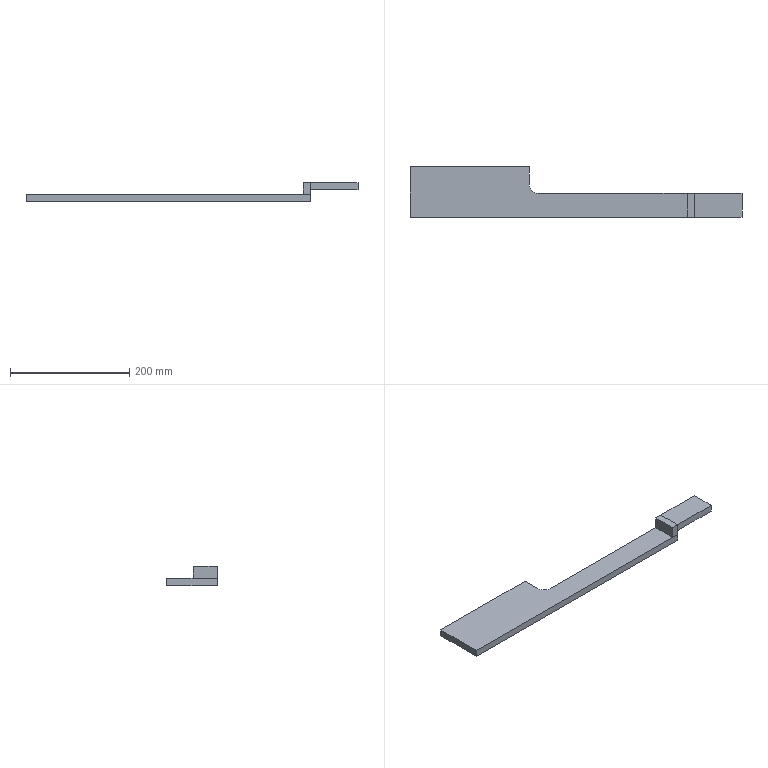Part | STEP file | PN_0035 | 1 solid | 17 faces | box 556.9 x 85 x 32 mm | volume 385323 mm3 | plane 16 | cylinder 1 | commonest cylinder face diameters 30 x1
STEP:
#1=CARTESIAN_POINT('',(0.,0.,0.));
#2=DIRECTION('',(0.,0.,1.));
#3=DIRECTION('',(1.,0.,0.));
#4=AXIS2_PLACEMENT_3D('',#1,#2,#3);
#5=CARTESIAN_POINT('',(238.4,-42.4,12.));
#6=VERTEX_POINT('',#5);
#7=CARTESIAN_POINT('',(238.4,-2.5,12.));
#8=VERTEX_POINT('',#7);
#9=CARTESIAN_POINT('',(238.4,42.4,12.));
#10=DIRECTION('',(0.,1.,0.));
#11=VECTOR('',#10,1.);
#12=LINE('',#9,#11);
#13=CARTESIAN_POINT('',(238.4,42.4,32.));
#14=DIRECTION('',(-1.,0.,0.));
#15=DIRECTION('',(0.,0.,1.));
#16=AXIS2_PLACEMENT_3D('',#13,#14,#15);
#17=PLANE('',#16);
#18=CARTESIAN_POINT('',(-20.,0.));
#19=DIRECTION('',(0.,1.));
#20=VECTOR('',#19,1.);
#21=LINE('',#18,#20);
#22=(GEOMETRIC_REPRESENTATION_CONTEXT(2)PARAMETRIC_REPRESENTATION_CONTEXT()REPRESENTATION_CONTEXT('',''));
#23=DEFINITIONAL_REPRESENTATION('',(#21),#22);
#24=PCURVE('',#17,#23);
#25=CARTESIAN_POINT('',(238.5,-42.5,12.));
#26=DIRECTION('',(0.,0.,1.));
#27=DIRECTION('',(1.,0.,0.));
#28=AXIS2_PLACEMENT_3D('',#25,#26,#27);
#29=PLANE('',#28);
#30=CARTESIAN_POINT('',(-0.1,84.9));
#31=DIRECTION('',(0.,1.));
#32=VECTOR('',#31,1.);
#33=LINE('',#30,#32);
#34=(GEOMETRIC_REPRESENTATION_CONTEXT(2)PARAMETRIC_REPRESENTATION_CONTEXT()REPRESENTATION_CONTEXT('',''));
#35=DEFINITIONAL_REPRESENTATION('',(#33),#34);
#36=PCURVE('',#29,#35);
#37=SURFACE_CURVE('',#12,(#24,#36),.PCURVE_S1.);
#38=EDGE_CURVE('',#6,#8,#37,.T.);
#39=ORIENTED_EDGE('',*,*,#38,.T.);
#40=CARTESIAN_POINT('',(238.4,-2.5,19.9));
#41=VERTEX_POINT('',#40);
#42=CARTESIAN_POINT('',(238.4,-2.5,32.));
#43=DIRECTION('',(0.,0.,1.));
#44=VECTOR('',#43,1.);
#45=LINE('',#42,#44);
#46=CARTESIAN_POINT('',(0.,-44.9));
#47=DIRECTION('',(1.,0.));
#48=VECTOR('',#47,1.);
#49=LINE('',#46,#48);
#50=(GEOMETRIC_REPRESENTATION_CONTEXT(2)PARAMETRIC_REPRESENTATION_CONTEXT()REPRESENTATION_CONTEXT('',''));
#51=DEFINITIONAL_REPRESENTATION('',(#49),#50);
#52=PCURVE('',#17,#51);
#53=CARTESIAN_POINT('',(-38.5,-2.5,32.));
#54=DIRECTION('',(0.,-1.,0.));
#55=DIRECTION('',(1.,0.,0.));
#56=AXIS2_PLACEMENT_3D('',#53,#54,#55);
#57=PLANE('',#56);
#58=CARTESIAN_POINT('',(276.9,0.));
#59=DIRECTION('',(0.,1.));
#60=VECTOR('',#59,1.);
#61=LINE('',#58,#60);
#62=(GEOMETRIC_REPRESENTATION_CONTEXT(2)PARAMETRIC_REPRESENTATION_CONTEXT()REPRESENTATION_CONTEXT('',''));
#63=DEFINITIONAL_REPRESENTATION('',(#61),#62);
#64=PCURVE('',#57,#63);
#65=SURFACE_CURVE('',#45,(#52,#64),.PCURVE_S1.);
#66=EDGE_CURVE('',#8,#41,#65,.T.);
#67=ORIENTED_EDGE('',*,*,#66,.T.);
#68=CARTESIAN_POINT('',(238.4,-42.3,19.9));
#69=VERTEX_POINT('',#68);
#70=CARTESIAN_POINT('',(238.4,42.3,19.9));
#71=DIRECTION('',(0.,1.,0.));
#72=VECTOR('',#71,1.);
#73=LINE('',#70,#72);
#74=CARTESIAN_POINT('',(-12.1,-0.1));
#75=DIRECTION('',(0.,1.));
#76=VECTOR('',#75,1.);
#77=LINE('',#74,#76);
#78=(GEOMETRIC_REPRESENTATION_CONTEXT(2)PARAMETRIC_REPRESENTATION_CONTEXT()REPRESENTATION_CONTEXT('',''));
#79=DEFINITIONAL_REPRESENTATION('',(#77),#78);
#80=PCURVE('',#17,#79);
#81=CARTESIAN_POINT('',(318.4,42.3,19.9));
#82=DIRECTION('',(0.,0.,1.));
#83=DIRECTION('',(0.,-1.,0.));
#84=AXIS2_PLACEMENT_3D('',#81,#82,#83);
#85=PLANE('',#84);
#86=CARTESIAN_POINT('',(0.,-80.));
#87=DIRECTION('',(-1.,0.));
#88=VECTOR('',#87,1.);
#89=LINE('',#86,#88);
#90=(GEOMETRIC_REPRESENTATION_CONTEXT(2)PARAMETRIC_REPRESENTATION_CONTEXT()REPRESENTATION_CONTEXT('',''));
#91=DEFINITIONAL_REPRESENTATION('',(#89),#90);
#92=PCURVE('',#85,#91);
#93=SURFACE_CURVE('',#73,(#80,#92),.PCURVE_S1.);
#94=EDGE_CURVE('',#69,#41,#93,.T.);
#95=ORIENTED_EDGE('',*,*,#94,.F.);
#96=CARTESIAN_POINT('',(238.4,-42.3,31.9));
#97=VERTEX_POINT('',#96);
#98=CARTESIAN_POINT('',(238.4,-42.3,31.9));
#99=DIRECTION('',(0.,0.,-1.));
#100=VECTOR('',#99,1.);
#101=LINE('',#98,#100);
#102=CARTESIAN_POINT('',(-0.1,-84.7));
#103=DIRECTION('',(-1.,0.));
#104=VECTOR('',#103,1.);
#105=LINE('',#102,#104);
#106=(GEOMETRIC_REPRESENTATION_CONTEXT(2)PARAMETRIC_REPRESENTATION_CONTEXT()REPRESENTATION_CONTEXT('',''));
#107=DEFINITIONAL_REPRESENTATION('',(#105),#106);
#108=PCURVE('',#17,#107);
#109=CARTESIAN_POINT('',(318.4,-42.3,31.9));
#110=DIRECTION('',(0.,1.,0.));
#111=DIRECTION('',(0.,0.,1.));
#112=AXIS2_PLACEMENT_3D('',#109,#110,#111);
#113=PLANE('',#112);
#114=CARTESIAN_POINT('',(0.,-80.));
#115=DIRECTION('',(-1.,0.));
#116=VECTOR('',#115,1.);
#117=LINE('',#114,#116);
#118=(GEOMETRIC_REPRESENTATION_CONTEXT(2)PARAMETRIC_REPRESENTATION_CONTEXT()REPRESENTATION_CONTEXT('',''));
#119=DEFINITIONAL_REPRESENTATION('',(#117),#118);
#120=PCURVE('',#113,#119);
#121=SURFACE_CURVE('',#101,(#108,#120),.PCURVE_S1.);
#122=EDGE_CURVE('',#97,#69,#121,.T.);
#123=ORIENTED_EDGE('',*,*,#122,.F.);
#124=CARTESIAN_POINT('',(238.4,-2.5,31.9));
#125=VERTEX_POINT('',#124);
#126=CARTESIAN_POINT('',(238.4,42.3,31.9));
#127=DIRECTION('',(0.,-1.,0.));
#128=VECTOR('',#127,1.);
#129=LINE('',#126,#128);
#130=CARTESIAN_POINT('',(-0.1,-0.1));
#131=DIRECTION('',(0.,-1.));
#132=VECTOR('',#131,1.);
#133=LINE('',#130,#132);
#134=(GEOMETRIC_REPRESENTATION_CONTEXT(2)PARAMETRIC_REPRESENTATION_CONTEXT()REPRESENTATION_CONTEXT('',''));
#135=DEFINITIONAL_REPRESENTATION('',(#133),#134);
#136=PCURVE('',#17,#135);
#137=CARTESIAN_POINT('',(318.4,42.3,31.9));
#138=DIRECTION('',(0.,0.,-1.));
#139=DIRECTION('',(0.,1.,0.));
#140=AXIS2_PLACEMENT_3D('',#137,#138,#139);
#141=PLANE('',#140);
#142=CARTESIAN_POINT('',(0.,-80.));
#143=DIRECTION('',(-1.,0.));
#144=VECTOR('',#143,1.);
#145=LINE('',#142,#144);
#146=(GEOMETRIC_REPRESENTATION_CONTEXT(2)PARAMETRIC_REPRESENTATION_CONTEXT()REPRESENTATION_CONTEXT('',''));
#147=DEFINITIONAL_REPRESENTATION('',(#145),#146);
#148=PCURVE('',#141,#147);
#149=SURFACE_CURVE('',#129,(#136,#148),.PCURVE_S1.);
#150=EDGE_CURVE('',#125,#97,#149,.T.);
#151=ORIENTED_EDGE('',*,*,#150,.F.);
#152=CARTESIAN_POINT('',(238.4,-2.5,32.));
#153=VERTEX_POINT('',#152);
#154=CARTESIAN_POINT('',(238.4,-2.5,32.));
#155=DIRECTION('',(0.,0.,1.));
#156=VECTOR('',#155,1.);
#157=LINE('',#154,#156);
#158=CARTESIAN_POINT('',(0.,-44.9));
#159=DIRECTION('',(1.,0.));
#160=VECTOR('',#159,1.);
#161=LINE('',#158,#160);
#162=(GEOMETRIC_REPRESENTATION_CONTEXT(2)PARAMETRIC_REPRESENTATION_CONTEXT()REPRESENTATION_CONTEXT('',''));
#163=DEFINITIONAL_REPRESENTATION('',(#161),#162);
#164=PCURVE('',#17,#163);
#165=CARTESIAN_POINT('',(276.9,0.));
#166=DIRECTION('',(0.,1.));
#167=VECTOR('',#166,1.);
#168=LINE('',#165,#167);
#169=(GEOMETRIC_REPRESENTATION_CONTEXT(2)PARAMETRIC_REPRESENTATION_CONTEXT()REPRESENTATION_CONTEXT('',''));
#170=DEFINITIONAL_REPRESENTATION('',(#168),#169);
#171=PCURVE('',#57,#170);
#172=SURFACE_CURVE('',#157,(#164,#171),.PCURVE_S1.);
#173=EDGE_CURVE('',#125,#153,#172,.T.);
#174=ORIENTED_EDGE('',*,*,#173,.T.);
#175=CARTESIAN_POINT('',(238.4,-42.4,32.));
#176=VERTEX_POINT('',#175);
#177=CARTESIAN_POINT('',(238.4,42.4,32.));
#178=DIRECTION('',(0.,1.,0.));
#179=VECTOR('',#178,1.);
#180=LINE('',#177,#179);
#181=CARTESIAN_POINT('',(0.,0.));
#182=DIRECTION('',(0.,1.));
#183=VECTOR('',#182,1.);
#184=LINE('',#181,#183);
#185=(GEOMETRIC_REPRESENTATION_CONTEXT(2)PARAMETRIC_REPRESENTATION_CONTEXT()REPRESENTATION_CONTEXT('',''));
#186=DEFINITIONAL_REPRESENTATION('',(#184),#185);
#187=PCURVE('',#17,#186);
#188=CARTESIAN_POINT('',(238.4,-42.4,32.));
#189=DIRECTION('',(0.,0.,-1.));
#190=DIRECTION('',(-1.,0.,0.));
#191=AXIS2_PLACEMENT_3D('',#188,#189,#190);
#192=PLANE('',#191);
#193=CARTESIAN_POINT('',(0.,84.8));
#194=DIRECTION('',(0.,1.));
#195=VECTOR('',#194,1.);
#196=LINE('',#193,#195);
#197=(GEOMETRIC_REPRESENTATION_CONTEXT(2)PARAMETRIC_REPRESENTATION_CONTEXT()REPRESENTATION_CONTEXT('',''));
#198=DEFINITIONAL_REPRESENTATION('',(#196),#197);
#199=PCURVE('',#192,#198);
#200=SURFACE_CURVE('',#180,(#187,#199),.PCURVE_S1.);
#201=EDGE_CURVE('',#176,#153,#200,.T.);
#202=ORIENTED_EDGE('',*,*,#201,.F.);
#203=CARTESIAN_POINT('',(238.4,-42.4,32.));
#204=DIRECTION('',(0.,0.,-1.));
#205=VECTOR('',#204,1.);
#206=LINE('',#203,#205);
#207=CARTESIAN_POINT('',(0.,-84.8));
#208=DIRECTION('',(-1.,0.));
#209=VECTOR('',#208,1.);
#210=LINE('',#207,#209);
#211=(GEOMETRIC_REPRESENTATION_CONTEXT(2)PARAMETRIC_REPRESENTATION_CONTEXT()REPRESENTATION_CONTEXT('',''));
#212=DEFINITIONAL_REPRESENTATION('',(#210),#211);
#213=PCURVE('',#17,#212);
#214=CARTESIAN_POINT('',(238.4,-42.4,32.));
#215=DIRECTION('',(0.,1.,0.));
#216=DIRECTION('',(0.,0.,1.));
#217=AXIS2_PLACEMENT_3D('',#214,#215,#216);
#218=PLANE('',#217);
#219=CARTESIAN_POINT('',(0.,0.));
#220=DIRECTION('',(-1.,0.));
#221=VECTOR('',#220,1.);
#222=LINE('',#219,#221);
#223=(GEOMETRIC_REPRESENTATION_CONTEXT(2)PARAMETRIC_REPRESENTATION_CONTEXT()REPRESENTATION_CONTEXT('',''));
#224=DEFINITIONAL_REPRESENTATION('',(#222),#223);
#225=PCURVE('',#218,#224);
#226=SURFACE_CURVE('',#206,(#213,#225),.PCURVE_S1.);
#227=EDGE_CURVE('',#176,#6,#226,.T.);
#228=ORIENTED_EDGE('',*,*,#227,.T.);
#229=EDGE_LOOP('',(#39,#67,#95,#123,#151,#174,#202,#228));
#230=FACE_BOUND('',#229,.T.);
#231=ADVANCED_FACE('',(#230),#17,.F.);
#232=CARTESIAN_POINT('',(-38.5,42.5,12.));
#233=VERTEX_POINT('',#232);
#234=CARTESIAN_POINT('',(-38.5,12.5,12.));
#235=VERTEX_POINT('',#234);
#236=CARTESIAN_POINT('',(-38.5,-42.5,12.));
#237=DIRECTION('',(0.,-1.,0.));
#238=VECTOR('',#237,1.);
#239=LINE('',#236,#238);
#240=CARTESIAN_POINT('',(-277.,0.));
#241=DIRECTION('',(0.,-1.));
#242=VECTOR('',#241,1.);
#243=LINE('',#240,#242);
#244=(GEOMETRIC_REPRESENTATION_CONTEXT(2)PARAMETRIC_REPRESENTATION_CONTEXT()REPRESENTATION_CONTEXT('',''));
#245=DEFINITIONAL_REPRESENTATION('',(#243),#244);
#246=PCURVE('',#29,#245);
#247=CARTESIAN_POINT('',(-38.5,42.5,32.));
#248=DIRECTION('',(-1.,0.,0.));
#249=DIRECTION('',(0.,-1.,0.));
#250=AXIS2_PLACEMENT_3D('',#247,#248,#249);
#251=PLANE('',#250);
#252=CARTESIAN_POINT('',(85.,-20.));
#253=DIRECTION('',(1.,0.));
#254=VECTOR('',#253,1.);
#255=LINE('',#252,#254);
#256=(GEOMETRIC_REPRESENTATION_CONTEXT(2)PARAMETRIC_REPRESENTATION_CONTEXT()REPRESENTATION_CONTEXT('',''));
#257=DEFINITIONAL_REPRESENTATION('',(#255),#256);
#258=PCURVE('',#251,#257);
#259=SURFACE_CURVE('',#239,(#246,#258),.PCURVE_S1.);
#260=EDGE_CURVE('',#233,#235,#259,.T.);
#261=ORIENTED_EDGE('',*,*,#260,.F.);
#262=CARTESIAN_POINT('',(-238.5,42.5,12.));
#263=VERTEX_POINT('',#262);
#264=CARTESIAN_POINT('',(-238.5,42.5,12.));
#265=DIRECTION('',(-1.,0.,0.));
#266=VECTOR('',#265,1.);
#267=LINE('',#264,#266);
#268=CARTESIAN_POINT('',(-477.,85.));
#269=DIRECTION('',(-1.,0.));
#270=VECTOR('',#269,1.);
#271=LINE('',#268,#270);
#272=(GEOMETRIC_REPRESENTATION_CONTEXT(2)PARAMETRIC_REPRESENTATION_CONTEXT()REPRESENTATION_CONTEXT('',''));
#273=DEFINITIONAL_REPRESENTATION('',(#271),#272);
#274=PCURVE('',#29,#273);
#275=CARTESIAN_POINT('',(-238.5,42.5,12.));
#276=DIRECTION('',(0.,-1.,0.));
#277=DIRECTION('',(0.,0.,-1.));
#278=AXIS2_PLACEMENT_3D('',#275,#276,#277);
#279=PLANE('',#278);
#280=CARTESIAN_POINT('',(0.,0.));
#281=DIRECTION('',(0.,-1.));
#282=VECTOR('',#281,1.);
#283=LINE('',#280,#282);
#284=(GEOMETRIC_REPRESENTATION_CONTEXT(2)PARAMETRIC_REPRESENTATION_CONTEXT()REPRESENTATION_CONTEXT('',''));
#285=DEFINITIONAL_REPRESENTATION('',(#283),#284);
#286=PCURVE('',#279,#285);
#287=SURFACE_CURVE('',#267,(#274,#286),.PCURVE_S1.);
#288=EDGE_CURVE('',#233,#263,#287,.T.);
#289=ORIENTED_EDGE('',*,*,#288,.T.);
#290=CARTESIAN_POINT('',(-238.5,-42.5,12.));
#291=VERTEX_POINT('',#290);
#292=CARTESIAN_POINT('',(-238.5,42.5,12.));
#293=DIRECTION('',(0.,-1.,0.));
#294=VECTOR('',#293,1.);
#295=LINE('',#292,#294);
#296=CARTESIAN_POINT('',(-477.,85.));
#297=DIRECTION('',(0.,-1.));
#298=VECTOR('',#297,1.);
#299=LINE('',#296,#298);
#300=(GEOMETRIC_REPRESENTATION_CONTEXT(2)PARAMETRIC_REPRESENTATION_CONTEXT()REPRESENTATION_CONTEXT('',''));
#301=DEFINITIONAL_REPRESENTATION('',(#299),#300);
#302=PCURVE('',#29,#301);
#303=CARTESIAN_POINT('',(-238.5,42.5,12.));
#304=DIRECTION('',(1.,0.,0.));
#305=DIRECTION('',(0.,0.,-1.));
#306=AXIS2_PLACEMENT_3D('',#303,#304,#305);
#307=PLANE('',#306);
#308=CARTESIAN_POINT('',(0.,0.));
#309=DIRECTION('',(0.,-1.));
#310=VECTOR('',#309,1.);
#311=LINE('',#308,#310);
#312=(GEOMETRIC_REPRESENTATION_CONTEXT(2)PARAMETRIC_REPRESENTATION_CONTEXT()REPRESENTATION_CONTEXT('',''));
#313=DEFINITIONAL_REPRESENTATION('',(#311),#312);
#314=PCURVE('',#307,#313);
#315=SURFACE_CURVE('',#295,(#302,#314),.PCURVE_S1.);
#316=EDGE_CURVE('',#263,#291,#315,.T.);
#317=ORIENTED_EDGE('',*,*,#316,.T.);
#318=CARTESIAN_POINT('',(238.5,-42.5,12.));
#319=VERTEX_POINT('',#318);
#320=CARTESIAN_POINT('',(-238.5,-42.5,12.));
#321=DIRECTION('',(1.,0.,0.));
#322=VECTOR('',#321,1.);
#323=LINE('',#320,#322);
#324=CARTESIAN_POINT('',(-477.,0.));
#325=DIRECTION('',(1.,0.));
#326=VECTOR('',#325,1.);
#327=LINE('',#324,#326);
#328=(GEOMETRIC_REPRESENTATION_CONTEXT(2)PARAMETRIC_REPRESENTATION_CONTEXT()REPRESENTATION_CONTEXT('',''));
#329=DEFINITIONAL_REPRESENTATION('',(#327),#328);
#330=PCURVE('',#29,#329);
#331=CARTESIAN_POINT('',(-238.5,-42.5,12.));
#332=DIRECTION('',(0.,1.,0.));
#333=DIRECTION('',(0.,0.,1.));
#334=AXIS2_PLACEMENT_3D('',#331,#332,#333);
#335=PLANE('',#334);
#336=CARTESIAN_POINT('',(0.,0.));
#337=DIRECTION('',(0.,1.));
#338=VECTOR('',#337,1.);
#339=LINE('',#336,#338);
#340=(GEOMETRIC_REPRESENTATION_CONTEXT(2)PARAMETRIC_REPRESENTATION_CONTEXT()REPRESENTATION_CONTEXT('',''));
#341=DEFINITIONAL_REPRESENTATION('',(#339),#340);
#342=PCURVE('',#335,#341);
#343=SURFACE_CURVE('',#323,(#330,#342),.PCURVE_S1.);
#344=EDGE_CURVE('',#291,#319,#343,.T.);
#345=ORIENTED_EDGE('',*,*,#344,.T.);
#346=CARTESIAN_POINT('',(238.5,-2.5,12.));
#347=VERTEX_POINT('',#346);
#348=CARTESIAN_POINT('',(238.5,42.5,12.));
#349=DIRECTION('',(0.,1.,0.));
#350=VECTOR('',#349,1.);
#351=LINE('',#348,#350);
#352=CARTESIAN_POINT('',(0.,85.));
#353=DIRECTION('',(0.,1.));
#354=VECTOR('',#353,1.);
#355=LINE('',#352,#354);
#356=(GEOMETRIC_REPRESENTATION_CONTEXT(2)PARAMETRIC_REPRESENTATION_CONTEXT()REPRESENTATION_CONTEXT('',''));
#357=DEFINITIONAL_REPRESENTATION('',(#355),#356);
#358=PCURVE('',#29,#357);
#359=CARTESIAN_POINT('',(238.5,42.5,12.));
#360=DIRECTION('',(-1.,0.,0.));
#361=DIRECTION('',(0.,-1.,0.));
#362=AXIS2_PLACEMENT_3D('',#359,#360,#361);
#363=PLANE('',#362);
#364=CARTESIAN_POINT('',(0.,0.));
#365=DIRECTION('',(-1.,0.));
#366=VECTOR('',#365,1.);
#367=LINE('',#364,#366);
#368=(GEOMETRIC_REPRESENTATION_CONTEXT(2)PARAMETRIC_REPRESENTATION_CONTEXT()REPRESENTATION_CONTEXT('',''));
#369=DEFINITIONAL_REPRESENTATION('',(#367),#368);
#370=PCURVE('',#363,#369);
#371=SURFACE_CURVE('',#351,(#358,#370),.PCURVE_S1.);
#372=EDGE_CURVE('',#319,#347,#371,.T.);
#373=ORIENTED_EDGE('',*,*,#372,.T.);
#374=CARTESIAN_POINT('',(238.5,-2.5,12.));
#375=DIRECTION('',(1.,0.,0.));
#376=VECTOR('',#375,1.);
#377=LINE('',#374,#376);
#378=CARTESIAN_POINT('',(0.,40.));
#379=DIRECTION('',(1.,0.));
#380=VECTOR('',#379,1.);
#381=LINE('',#378,#380);
#382=(GEOMETRIC_REPRESENTATION_CONTEXT(2)PARAMETRIC_REPRESENTATION_CONTEXT()REPRESENTATION_CONTEXT('',''));
#383=DEFINITIONAL_REPRESENTATION('',(#381),#382);
#384=PCURVE('',#29,#383);
#385=CARTESIAN_POINT('',(277.,-20.));
#386=DIRECTION('',(1.,0.));
#387=VECTOR('',#386,1.);
#388=LINE('',#385,#387);
#389=(GEOMETRIC_REPRESENTATION_CONTEXT(2)PARAMETRIC_REPRESENTATION_CONTEXT()REPRESENTATION_CONTEXT('',''));
#390=DEFINITIONAL_REPRESENTATION('',(#388),#389);
#391=PCURVE('',#57,#390);
#392=SURFACE_CURVE('',#377,(#384,#391),.PCURVE_S1.);
#393=EDGE_CURVE('',#8,#347,#392,.T.);
#394=ORIENTED_EDGE('',*,*,#393,.F.);
#395=ORIENTED_EDGE('',*,*,#38,.F.);
#396=CARTESIAN_POINT('',(226.4,-42.4,12.));
#397=VERTEX_POINT('',#396);
#398=CARTESIAN_POINT('',(238.4,-42.4,12.));
#399=DIRECTION('',(1.,0.,0.));
#400=VECTOR('',#399,1.);
#401=LINE('',#398,#400);
#402=CARTESIAN_POINT('',(-0.1,0.1));
#403=DIRECTION('',(1.,0.));
#404=VECTOR('',#403,1.);
#405=LINE('',#402,#404);
#406=(GEOMETRIC_REPRESENTATION_CONTEXT(2)PARAMETRIC_REPRESENTATION_CONTEXT()REPRESENTATION_CONTEXT('',''));
#407=DEFINITIONAL_REPRESENTATION('',(#405),#406);
#408=PCURVE('',#29,#407);
#409=CARTESIAN_POINT('',(-20.,0.));
#410=DIRECTION('',(0.,1.));
#411=VECTOR('',#410,1.);
#412=LINE('',#409,#411);
#413=(GEOMETRIC_REPRESENTATION_CONTEXT(2)PARAMETRIC_REPRESENTATION_CONTEXT()REPRESENTATION_CONTEXT('',''));
#414=DEFINITIONAL_REPRESENTATION('',(#412),#413);
#415=PCURVE('',#218,#414);
#416=SURFACE_CURVE('',#401,(#408,#415),.PCURVE_S1.);
#417=EDGE_CURVE('',#397,#6,#416,.T.);
#418=ORIENTED_EDGE('',*,*,#417,.F.);
#419=CARTESIAN_POINT('',(226.4,-2.5,12.));
#420=VERTEX_POINT('',#419);
#421=CARTESIAN_POINT('',(226.4,42.4,12.));
#422=DIRECTION('',(0.,-1.,0.));
#423=VECTOR('',#422,1.);
#424=LINE('',#421,#423);
#425=CARTESIAN_POINT('',(-12.1,84.9));
#426=DIRECTION('',(0.,-1.));
#427=VECTOR('',#426,1.);
#428=LINE('',#425,#427);
#429=(GEOMETRIC_REPRESENTATION_CONTEXT(2)PARAMETRIC_REPRESENTATION_CONTEXT()REPRESENTATION_CONTEXT('',''));
#430=DEFINITIONAL_REPRESENTATION('',(#428),#429);
#431=PCURVE('',#29,#430);
#432=CARTESIAN_POINT('',(226.4,42.4,32.));
#433=DIRECTION('',(1.,0.,0.));
#434=DIRECTION('',(0.,0.,-1.));
#435=AXIS2_PLACEMENT_3D('',#432,#433,#434);
#436=PLANE('',#435);
#437=CARTESIAN_POINT('',(20.,0.));
#438=DIRECTION('',(0.,-1.));
#439=VECTOR('',#438,1.);
#440=LINE('',#437,#439);
#441=(GEOMETRIC_REPRESENTATION_CONTEXT(2)PARAMETRIC_REPRESENTATION_CONTEXT()REPRESENTATION_CONTEXT('',''));
#442=DEFINITIONAL_REPRESENTATION('',(#440),#441);
#443=PCURVE('',#436,#442);
#444=SURFACE_CURVE('',#424,(#431,#443),.PCURVE_S1.);
#445=EDGE_CURVE('',#420,#397,#444,.T.);
#446=ORIENTED_EDGE('',*,*,#445,.F.);
#447=CARTESIAN_POINT('',(-23.5,-2.5,12.));
#448=VERTEX_POINT('',#447);
#449=CARTESIAN_POINT('',(238.5,-2.5,12.));
#450=DIRECTION('',(1.,0.,0.));
#451=VECTOR('',#450,1.);
#452=LINE('',#449,#451);
#453=CARTESIAN_POINT('',(0.,40.));
#454=DIRECTION('',(1.,0.));
#455=VECTOR('',#454,1.);
#456=LINE('',#453,#455);
#457=(GEOMETRIC_REPRESENTATION_CONTEXT(2)PARAMETRIC_REPRESENTATION_CONTEXT()REPRESENTATION_CONTEXT('',''));
#458=DEFINITIONAL_REPRESENTATION('',(#456),#457);
#459=PCURVE('',#29,#458);
#460=CARTESIAN_POINT('',(277.,-20.));
#461=DIRECTION('',(1.,0.));
#462=VECTOR('',#461,1.);
#463=LINE('',#460,#462);
#464=(GEOMETRIC_REPRESENTATION_CONTEXT(2)PARAMETRIC_REPRESENTATION_CONTEXT()REPRESENTATION_CONTEXT('',''));
#465=DEFINITIONAL_REPRESENTATION('',(#463),#464);
#466=PCURVE('',#57,#465);
#467=SURFACE_CURVE('',#452,(#459,#466),.PCURVE_S1.);
#468=EDGE_CURVE('',#448,#420,#467,.T.);
#469=ORIENTED_EDGE('',*,*,#468,.F.);
#470=CARTESIAN_POINT('',(-23.5,12.5,12.));
#471=DIRECTION('',(0.,0.,-1.));
#472=DIRECTION('',(1.,0.,0.));
#473=AXIS2_PLACEMENT_3D('',#470,#471,#472);
#474=CIRCLE('',#473,15.);
#475=CARTESIAN_POINT('',(-247.,55.));
#476=CARTESIAN_POINT('',(-247.,29.019));
#477=CARTESIAN_POINT('',(-269.5,42.01));
#478=CARTESIAN_POINT('',(-292.,55.));
#479=CARTESIAN_POINT('',(-269.5,67.99));
#480=CARTESIAN_POINT('',(-247.,80.981));
#481=CARTESIAN_POINT('',(-247.,55.));
#482=(BOUNDED_CURVE()B_SPLINE_CURVE(2,(#475,#476,#477,#478,#479,#480,#481),.UNSPECIFIED.,.T.,.F.)B_SPLINE_CURVE_WITH_KNOTS((1,2,2,2,2,1),(-2.094,0.,2.094,4.189,6.283,8.378),.UNSPECIFIED.)CURVE()GEOMETRIC_REPRESENTATION_ITEM()RATIONAL_B_SPLINE_CURVE((1.,0.5,1.,0.5,1.,0.5,1.))REPRESENTATION_ITEM(''));
#483=(GEOMETRIC_REPRESENTATION_CONTEXT(2)PARAMETRIC_REPRESENTATION_CONTEXT()REPRESENTATION_CONTEXT('',''));
#484=DEFINITIONAL_REPRESENTATION('',(#482),#483);
#485=PCURVE('',#29,#484);
#486=CARTESIAN_POINT('',(-23.5,12.5,32.));
#487=DIRECTION('',(0.,0.,1.));
#488=DIRECTION('',(1.,0.,0.));
#489=AXIS2_PLACEMENT_3D('',#486,#487,#488);
#490=CYLINDRICAL_SURFACE('',#489,15.);
#491=CARTESIAN_POINT('',(6.283,-20.));
#492=DIRECTION('',(-1.,0.));
#493=VECTOR('',#492,1.);
#494=LINE('',#491,#493);
#495=(GEOMETRIC_REPRESENTATION_CONTEXT(2)PARAMETRIC_REPRESENTATION_CONTEXT()REPRESENTATION_CONTEXT('',''));
#496=DEFINITIONAL_REPRESENTATION('',(#494),#495);
#497=PCURVE('',#490,#496);
#498=SURFACE_CURVE('',#474,(#485,#497),.PCURVE_S1.);
#499=EDGE_CURVE('',#448,#235,#498,.T.);
#500=ORIENTED_EDGE('',*,*,#499,.T.);
#501=EDGE_LOOP('',(#261,#289,#317,#345,#373,#394,#395,#418,#446,#469,#500));
#502=FACE_BOUND('',#501,.T.);
#503=ADVANCED_FACE('',(#502),#29,.T.);
#504=CARTESIAN_POINT('',(238.5,-42.5,0.));
#505=VERTEX_POINT('',#504);
#506=CARTESIAN_POINT('',(238.5,-2.5,0.));
#507=VERTEX_POINT('',#506);
#508=CARTESIAN_POINT('',(238.5,42.5,0.));
#509=DIRECTION('',(0.,1.,0.));
#510=VECTOR('',#509,1.);
#511=LINE('',#508,#510);
#512=CARTESIAN_POINT('',(0.,-12.));
#513=DIRECTION('',(-1.,0.));
#514=VECTOR('',#513,1.);
#515=LINE('',#512,#514);
#516=(GEOMETRIC_REPRESENTATION_CONTEXT(2)PARAMETRIC_REPRESENTATION_CONTEXT()REPRESENTATION_CONTEXT('',''));
#517=DEFINITIONAL_REPRESENTATION('',(#515),#516);
#518=PCURVE('',#363,#517);
#519=CARTESIAN_POINT('',(238.5,-42.5,0.));
#520=DIRECTION('',(0.,0.,1.));
#521=DIRECTION('',(1.,0.,0.));
#522=AXIS2_PLACEMENT_3D('',#519,#520,#521);
#523=PLANE('',#522);
#524=CARTESIAN_POINT('',(0.,85.));
#525=DIRECTION('',(0.,1.));
#526=VECTOR('',#525,1.);
#527=LINE('',#524,#526);
#528=(GEOMETRIC_REPRESENTATION_CONTEXT(2)PARAMETRIC_REPRESENTATION_CONTEXT()REPRESENTATION_CONTEXT('',''));
#529=DEFINITIONAL_REPRESENTATION('',(#527),#528);
#530=PCURVE('',#523,#529);
#531=SURFACE_CURVE('',#511,(#518,#530),.PCURVE_S1.);
#532=EDGE_CURVE('',#505,#507,#531,.T.);
#533=ORIENTED_EDGE('',*,*,#532,.T.);
#534=CARTESIAN_POINT('',(238.5,-2.5,12.));
#535=DIRECTION('',(0.,0.,1.));
#536=VECTOR('',#535,1.);
#537=LINE('',#534,#536);
#538=CARTESIAN_POINT('',(45.,0.));
#539=DIRECTION('',(0.,1.));
#540=VECTOR('',#539,1.);
#541=LINE('',#538,#540);
#542=(GEOMETRIC_REPRESENTATION_CONTEXT(2)PARAMETRIC_REPRESENTATION_CONTEXT()REPRESENTATION_CONTEXT('',''));
#543=DEFINITIONAL_REPRESENTATION('',(#541),#542);
#544=PCURVE('',#363,#543);
#545=CARTESIAN_POINT('',(277.,-20.));
#546=DIRECTION('',(0.,1.));
#547=VECTOR('',#546,1.);
#548=LINE('',#545,#547);
#549=(GEOMETRIC_REPRESENTATION_CONTEXT(2)PARAMETRIC_REPRESENTATION_CONTEXT()REPRESENTATION_CONTEXT('',''));
#550=DEFINITIONAL_REPRESENTATION('',(#548),#549);
#551=PCURVE('',#57,#550);
#552=SURFACE_CURVE('',#537,(#544,#551),.PCURVE_S1.);
#553=EDGE_CURVE('',#507,#347,#552,.T.);
#554=ORIENTED_EDGE('',*,*,#553,.T.);
#555=ORIENTED_EDGE('',*,*,#372,.F.);
#556=CARTESIAN_POINT('',(238.5,-42.5,12.));
#557=DIRECTION('',(0.,0.,-1.));
#558=VECTOR('',#557,1.);
#559=LINE('',#556,#558);
#560=CARTESIAN_POINT('',(85.,0.));
#561=DIRECTION('',(0.,-1.));
#562=VECTOR('',#561,1.);
#563=LINE('',#560,#562);
#564=(GEOMETRIC_REPRESENTATION_CONTEXT(2)PARAMETRIC_REPRESENTATION_CONTEXT()REPRESENTATION_CONTEXT('',''));
#565=DEFINITIONAL_REPRESENTATION('',(#563),#564);
#566=PCURVE('',#363,#565);
#567=CARTESIAN_POINT('',(0.,477.));
#568=DIRECTION('',(-1.,0.));
#569=VECTOR('',#568,1.);
#570=LINE('',#567,#569);
#571=(GEOMETRIC_REPRESENTATION_CONTEXT(2)PARAMETRIC_REPRESENTATION_CONTEXT()REPRESENTATION_CONTEXT('',''));
#572=DEFINITIONAL_REPRESENTATION('',(#570),#571);
#573=PCURVE('',#335,#572);
#574=SURFACE_CURVE('',#559,(#566,#573),.PCURVE_S1.);
#575=EDGE_CURVE('',#319,#505,#574,.T.);
#576=ORIENTED_EDGE('',*,*,#575,.T.);
#577=EDGE_LOOP('',(#533,#554,#555,#576));
#578=FACE_BOUND('',#577,.T.);
#579=ADVANCED_FACE('',(#578),#363,.F.);
#580=ORIENTED_EDGE('',*,*,#288,.F.);
#581=CARTESIAN_POINT('',(-38.5,42.5,0.));
#582=VERTEX_POINT('',#581);
#583=CARTESIAN_POINT('',(-38.5,42.5,32.));
#584=DIRECTION('',(0.,0.,-1.));
#585=VECTOR('',#584,1.);
#586=LINE('',#583,#585);
#587=CARTESIAN_POINT('',(-20.,200.));
#588=DIRECTION('',(1.,0.));
#589=VECTOR('',#588,1.);
#590=LINE('',#587,#589);
#591=(GEOMETRIC_REPRESENTATION_CONTEXT(2)PARAMETRIC_REPRESENTATION_CONTEXT()REPRESENTATION_CONTEXT('',''));
#592=DEFINITIONAL_REPRESENTATION('',(#590),#591);
#593=PCURVE('',#279,#592);
#594=CARTESIAN_POINT('',(0.,0.));
#595=DIRECTION('',(0.,-1.));
#596=VECTOR('',#595,1.);
#597=LINE('',#594,#596);
#598=(GEOMETRIC_REPRESENTATION_CONTEXT(2)PARAMETRIC_REPRESENTATION_CONTEXT()REPRESENTATION_CONTEXT('',''));
#599=DEFINITIONAL_REPRESENTATION('',(#597),#598);
#600=PCURVE('',#251,#599);
#601=SURFACE_CURVE('',#586,(#593,#600),.PCURVE_S1.);
#602=EDGE_CURVE('',#233,#582,#601,.T.);
#603=ORIENTED_EDGE('',*,*,#602,.T.);
#604=CARTESIAN_POINT('',(-238.5,42.5,0.));
#605=VERTEX_POINT('',#604);
#606=CARTESIAN_POINT('',(-238.5,42.5,0.));
#607=DIRECTION('',(-1.,0.,0.));
#608=VECTOR('',#607,1.);
#609=LINE('',#606,#608);
#610=CARTESIAN_POINT('',(12.,0.));
#611=DIRECTION('',(0.,-1.));
#612=VECTOR('',#611,1.);
#613=LINE('',#610,#612);
#614=(GEOMETRIC_REPRESENTATION_CONTEXT(2)PARAMETRIC_REPRESENTATION_CONTEXT()REPRESENTATION_CONTEXT('',''));
#615=DEFINITIONAL_REPRESENTATION('',(#613),#614);
#616=PCURVE('',#279,#615);
#617=CARTESIAN_POINT('',(-477.,85.));
#618=DIRECTION('',(-1.,0.));
#619=VECTOR('',#618,1.);
#620=LINE('',#617,#619);
#621=(GEOMETRIC_REPRESENTATION_CONTEXT(2)PARAMETRIC_REPRESENTATION_CONTEXT()REPRESENTATION_CONTEXT('',''));
#622=DEFINITIONAL_REPRESENTATION('',(#620),#621);
#623=PCURVE('',#523,#622);
#624=SURFACE_CURVE('',#609,(#616,#623),.PCURVE_S1.);
#625=EDGE_CURVE('',#582,#605,#624,.T.);
#626=ORIENTED_EDGE('',*,*,#625,.T.);
#627=CARTESIAN_POINT('',(-238.5,42.5,12.));
#628=DIRECTION('',(0.,0.,-1.));
#629=VECTOR('',#628,1.);
#630=LINE('',#627,#629);
#631=CARTESIAN_POINT('',(0.,0.));
#632=DIRECTION('',(1.,0.));
#633=VECTOR('',#632,1.);
#634=LINE('',#631,#633);
#635=(GEOMETRIC_REPRESENTATION_CONTEXT(2)PARAMETRIC_REPRESENTATION_CONTEXT()REPRESENTATION_CONTEXT('',''));
#636=DEFINITIONAL_REPRESENTATION('',(#634),#635);
#637=PCURVE('',#279,#636);
#638=CARTESIAN_POINT('',(0.,0.));
#639=DIRECTION('',(1.,0.));
#640=VECTOR('',#639,1.);
#641=LINE('',#638,#640);
#642=(GEOMETRIC_REPRESENTATION_CONTEXT(2)PARAMETRIC_REPRESENTATION_CONTEXT()REPRESENTATION_CONTEXT('',''));
#643=DEFINITIONAL_REPRESENTATION('',(#641),#642);
#644=PCURVE('',#307,#643);
#645=SURFACE_CURVE('',#630,(#637,#644),.PCURVE_S1.);
#646=EDGE_CURVE('',#263,#605,#645,.T.);
#647=ORIENTED_EDGE('',*,*,#646,.F.);
#648=EDGE_LOOP('',(#580,#603,#626,#647));
#649=FACE_BOUND('',#648,.T.);
#650=ADVANCED_FACE('',(#649),#279,.F.);
#651=CARTESIAN_POINT('',(-238.5,-42.5,0.));
#652=VERTEX_POINT('',#651);
#653=CARTESIAN_POINT('',(-238.5,42.5,0.));
#654=DIRECTION('',(0.,-1.,0.));
#655=VECTOR('',#654,1.);
#656=LINE('',#653,#655);
#657=CARTESIAN_POINT('',(12.,0.));
#658=DIRECTION('',(0.,-1.));
#659=VECTOR('',#658,1.);
#660=LINE('',#657,#659);
#661=(GEOMETRIC_REPRESENTATION_CONTEXT(2)PARAMETRIC_REPRESENTATION_CONTEXT()REPRESENTATION_CONTEXT('',''));
#662=DEFINITIONAL_REPRESENTATION('',(#660),#661);
#663=PCURVE('',#307,#662);
#664=CARTESIAN_POINT('',(-477.,85.));
#665=DIRECTION('',(0.,-1.));
#666=VECTOR('',#665,1.);
#667=LINE('',#664,#666);
#668=(GEOMETRIC_REPRESENTATION_CONTEXT(2)PARAMETRIC_REPRESENTATION_CONTEXT()REPRESENTATION_CONTEXT('',''));
#669=DEFINITIONAL_REPRESENTATION('',(#667),#668);
#670=PCURVE('',#523,#669);
#671=SURFACE_CURVE('',#656,(#663,#670),.PCURVE_S1.);
#672=EDGE_CURVE('',#605,#652,#671,.T.);
#673=ORIENTED_EDGE('',*,*,#672,.T.);
#674=CARTESIAN_POINT('',(-238.5,-42.5,12.));
#675=DIRECTION('',(0.,0.,-1.));
#676=VECTOR('',#675,1.);
#677=LINE('',#674,#676);
#678=CARTESIAN_POINT('',(0.,-85.));
#679=DIRECTION('',(1.,0.));
#680=VECTOR('',#679,1.);
#681=LINE('',#678,#680);
#682=(GEOMETRIC_REPRESENTATION_CONTEXT(2)PARAMETRIC_REPRESENTATION_CONTEXT()REPRESENTATION_CONTEXT('',''));
#683=DEFINITIONAL_REPRESENTATION('',(#681),#682);
#684=PCURVE('',#307,#683);
#685=CARTESIAN_POINT('',(0.,0.));
#686=DIRECTION('',(-1.,0.));
#687=VECTOR('',#686,1.);
#688=LINE('',#685,#687);
#689=(GEOMETRIC_REPRESENTATION_CONTEXT(2)PARAMETRIC_REPRESENTATION_CONTEXT()REPRESENTATION_CONTEXT('',''));
#690=DEFINITIONAL_REPRESENTATION('',(#688),#689);
#691=PCURVE('',#335,#690);
#692=SURFACE_CURVE('',#677,(#684,#691),.PCURVE_S1.);
#693=EDGE_CURVE('',#291,#652,#692,.T.);
#694=ORIENTED_EDGE('',*,*,#693,.F.);
#695=ORIENTED_EDGE('',*,*,#316,.F.);
#696=ORIENTED_EDGE('',*,*,#646,.T.);
#697=EDGE_LOOP('',(#673,#694,#695,#696));
#698=FACE_BOUND('',#697,.T.);
#699=ADVANCED_FACE('',(#698),#307,.F.);
#700=CARTESIAN_POINT('',(-238.5,-42.5,0.));
#701=DIRECTION('',(1.,0.,0.));
#702=VECTOR('',#701,1.);
#703=LINE('',#700,#702);
#704=CARTESIAN_POINT('',(-12.,0.));
#705=DIRECTION('',(0.,1.));
#706=VECTOR('',#705,1.);
#707=LINE('',#704,#706);
#708=(GEOMETRIC_REPRESENTATION_CONTEXT(2)PARAMETRIC_REPRESENTATION_CONTEXT()REPRESENTATION_CONTEXT('',''));
#709=DEFINITIONAL_REPRESENTATION('',(#707),#708);
#710=PCURVE('',#335,#709);
#711=CARTESIAN_POINT('',(-477.,0.));
#712=DIRECTION('',(1.,0.));
#713=VECTOR('',#712,1.);
#714=LINE('',#711,#713);
#715=(GEOMETRIC_REPRESENTATION_CONTEXT(2)PARAMETRIC_REPRESENTATION_CONTEXT()REPRESENTATION_CONTEXT('',''));
#716=DEFINITIONAL_REPRESENTATION('',(#714),#715);
#717=PCURVE('',#523,#716);
#718=SURFACE_CURVE('',#703,(#710,#717),.PCURVE_S1.);
#719=EDGE_CURVE('',#652,#505,#718,.T.);
#720=ORIENTED_EDGE('',*,*,#719,.T.);
#721=ORIENTED_EDGE('',*,*,#575,.F.);
#722=ORIENTED_EDGE('',*,*,#344,.F.);
#723=ORIENTED_EDGE('',*,*,#693,.T.);
#724=EDGE_LOOP('',(#720,#721,#722,#723));
#725=FACE_BOUND('',#724,.T.);
#726=ADVANCED_FACE('',(#725),#335,.F.);
#727=ORIENTED_EDGE('',*,*,#625,.F.);
#728=CARTESIAN_POINT('',(-38.5,12.5,0.));
#729=VERTEX_POINT('',#728);
#730=CARTESIAN_POINT('',(-38.5,42.5,0.));
#731=DIRECTION('',(0.,1.,0.));
#732=VECTOR('',#731,1.);
#733=LINE('',#730,#732);
#734=CARTESIAN_POINT('',(-277.,85.));
#735=DIRECTION('',(0.,1.));
#736=VECTOR('',#735,1.);
#737=LINE('',#734,#736);
#738=(GEOMETRIC_REPRESENTATION_CONTEXT(2)PARAMETRIC_REPRESENTATION_CONTEXT()REPRESENTATION_CONTEXT('',''));
#739=DEFINITIONAL_REPRESENTATION('',(#737),#738);
#740=PCURVE('',#523,#739);
#741=CARTESIAN_POINT('',(0.,-32.));
#742=DIRECTION('',(-1.,0.));
#743=VECTOR('',#742,1.);
#744=LINE('',#741,#743);
#745=(GEOMETRIC_REPRESENTATION_CONTEXT(2)PARAMETRIC_REPRESENTATION_CONTEXT()REPRESENTATION_CONTEXT('',''));
#746=DEFINITIONAL_REPRESENTATION('',(#744),#745);
#747=PCURVE('',#251,#746);
#748=SURFACE_CURVE('',#733,(#740,#747),.PCURVE_S1.);
#749=EDGE_CURVE('',#729,#582,#748,.T.);
#750=ORIENTED_EDGE('',*,*,#749,.F.);
#751=CARTESIAN_POINT('',(-23.5,-2.5,0.));
#752=VERTEX_POINT('',#751);
#753=CARTESIAN_POINT('',(-23.5,12.5,0.));
#754=DIRECTION('',(0.,0.,1.));
#755=DIRECTION('',(1.,0.,0.));
#756=AXIS2_PLACEMENT_3D('',#753,#754,#755);
#757=CIRCLE('',#756,15.);
#758=CARTESIAN_POINT('',(-262.,55.));
#759=DIRECTION('',(1.,0.));
#760=AXIS2_PLACEMENT_2D('',#758,#759);
#761=CIRCLE('',#760,15.);
#762=(GEOMETRIC_REPRESENTATION_CONTEXT(2)PARAMETRIC_REPRESENTATION_CONTEXT()REPRESENTATION_CONTEXT('',''));
#763=DEFINITIONAL_REPRESENTATION('',(#761),#762);
#764=PCURVE('',#523,#763);
#765=CARTESIAN_POINT('',(0.,-32.));
#766=DIRECTION('',(1.,0.));
#767=VECTOR('',#766,1.);
#768=LINE('',#765,#767);
#769=(GEOMETRIC_REPRESENTATION_CONTEXT(2)PARAMETRIC_REPRESENTATION_CONTEXT()REPRESENTATION_CONTEXT('',''));
#770=DEFINITIONAL_REPRESENTATION('',(#768),#769);
#771=PCURVE('',#490,#770);
#772=SURFACE_CURVE('',#757,(#764,#771),.PCURVE_S1.);
#773=EDGE_CURVE('',#729,#752,#772,.T.);
#774=ORIENTED_EDGE('',*,*,#773,.T.);
#775=CARTESIAN_POINT('',(-38.5,-2.5,0.));
#776=DIRECTION('',(-1.,0.,0.));
#777=VECTOR('',#776,1.);
#778=LINE('',#775,#777);
#779=CARTESIAN_POINT('',(-277.,40.));
#780=DIRECTION('',(-1.,0.));
#781=VECTOR('',#780,1.);
#782=LINE('',#779,#781);
#783=(GEOMETRIC_REPRESENTATION_CONTEXT(2)PARAMETRIC_REPRESENTATION_CONTEXT()REPRESENTATION_CONTEXT('',''));
#784=DEFINITIONAL_REPRESENTATION('',(#782),#783);
#785=PCURVE('',#523,#784);
#786=CARTESIAN_POINT('',(0.,-32.));
#787=DIRECTION('',(-1.,0.));
#788=VECTOR('',#787,1.);
#789=LINE('',#786,#788);
#790=(GEOMETRIC_REPRESENTATION_CONTEXT(2)PARAMETRIC_REPRESENTATION_CONTEXT()REPRESENTATION_CONTEXT('',''));
#791=DEFINITIONAL_REPRESENTATION('',(#789),#790);
#792=PCURVE('',#57,#791);
#793=SURFACE_CURVE('',#778,(#785,#792),.PCURVE_S1.);
#794=EDGE_CURVE('',#507,#752,#793,.T.);
#795=ORIENTED_EDGE('',*,*,#794,.F.);
#796=ORIENTED_EDGE('',*,*,#532,.F.);
#797=ORIENTED_EDGE('',*,*,#719,.F.);
#798=ORIENTED_EDGE('',*,*,#672,.F.);
#799=EDGE_LOOP('',(#727,#750,#774,#795,#796,#797,#798));
#800=FACE_BOUND('',#799,.T.);
#801=ADVANCED_FACE('',(#800),#523,.F.);
#802=CARTESIAN_POINT('',(226.4,-2.5,32.));
#803=VERTEX_POINT('',#802);
#804=CARTESIAN_POINT('',(226.4,-42.4,32.));
#805=VERTEX_POINT('',#804);
#806=CARTESIAN_POINT('',(226.4,42.4,32.));
#807=DIRECTION('',(0.,-1.,0.));
#808=VECTOR('',#807,1.);
#809=LINE('',#806,#808);
#810=CARTESIAN_POINT('',(0.,0.));
#811=DIRECTION('',(0.,-1.));
#812=VECTOR('',#811,1.);
#813=LINE('',#810,#812);
#814=(GEOMETRIC_REPRESENTATION_CONTEXT(2)PARAMETRIC_REPRESENTATION_CONTEXT()REPRESENTATION_CONTEXT('',''));
#815=DEFINITIONAL_REPRESENTATION('',(#813),#814);
#816=PCURVE('',#436,#815);
#817=CARTESIAN_POINT('',(12.,84.8));
#818=DIRECTION('',(0.,-1.));
#819=VECTOR('',#818,1.);
#820=LINE('',#817,#819);
#821=(GEOMETRIC_REPRESENTATION_CONTEXT(2)PARAMETRIC_REPRESENTATION_CONTEXT()REPRESENTATION_CONTEXT('',''));
#822=DEFINITIONAL_REPRESENTATION('',(#820),#821);
#823=PCURVE('',#192,#822);
#824=SURFACE_CURVE('',#809,(#816,#823),.PCURVE_S1.);
#825=EDGE_CURVE('',#803,#805,#824,.T.);
#826=ORIENTED_EDGE('',*,*,#825,.F.);
#827=CARTESIAN_POINT('',(226.4,-2.5,32.));
#828=DIRECTION('',(0.,0.,-1.));
#829=VECTOR('',#828,1.);
#830=LINE('',#827,#829);
#831=CARTESIAN_POINT('',(0.,-44.9));
#832=DIRECTION('',(1.,0.));
#833=VECTOR('',#832,1.);
#834=LINE('',#831,#833);
#835=(GEOMETRIC_REPRESENTATION_CONTEXT(2)PARAMETRIC_REPRESENTATION_CONTEXT()REPRESENTATION_CONTEXT('',''));
#836=DEFINITIONAL_REPRESENTATION('',(#834),#835);
#837=PCURVE('',#436,#836);
#838=CARTESIAN_POINT('',(264.9,0.));
#839=DIRECTION('',(0.,-1.));
#840=VECTOR('',#839,1.);
#841=LINE('',#838,#840);
#842=(GEOMETRIC_REPRESENTATION_CONTEXT(2)PARAMETRIC_REPRESENTATION_CONTEXT()REPRESENTATION_CONTEXT('',''));
#843=DEFINITIONAL_REPRESENTATION('',(#841),#842);
#844=PCURVE('',#57,#843);
#845=SURFACE_CURVE('',#830,(#837,#844),.PCURVE_S1.);
#846=EDGE_CURVE('',#803,#420,#845,.T.);
#847=ORIENTED_EDGE('',*,*,#846,.T.);
#848=ORIENTED_EDGE('',*,*,#445,.T.);
#849=CARTESIAN_POINT('',(226.4,-42.4,32.));
#850=DIRECTION('',(0.,0.,-1.));
#851=VECTOR('',#850,1.);
#852=LINE('',#849,#851);
#853=CARTESIAN_POINT('',(0.,-84.8));
#854=DIRECTION('',(1.,0.));
#855=VECTOR('',#854,1.);
#856=LINE('',#853,#855);
#857=(GEOMETRIC_REPRESENTATION_CONTEXT(2)PARAMETRIC_REPRESENTATION_CONTEXT()REPRESENTATION_CONTEXT('',''));
#858=DEFINITIONAL_REPRESENTATION('',(#856),#857);
#859=PCURVE('',#436,#858);
#860=CARTESIAN_POINT('',(0.,-12.));
#861=DIRECTION('',(-1.,0.));
#862=VECTOR('',#861,1.);
#863=LINE('',#860,#862);
#864=(GEOMETRIC_REPRESENTATION_CONTEXT(2)PARAMETRIC_REPRESENTATION_CONTEXT()REPRESENTATION_CONTEXT('',''));
#865=DEFINITIONAL_REPRESENTATION('',(#863),#864);
#866=PCURVE('',#218,#865);
#867=SURFACE_CURVE('',#852,(#859,#866),.PCURVE_S1.);
#868=EDGE_CURVE('',#805,#397,#867,.T.);
#869=ORIENTED_EDGE('',*,*,#868,.F.);
#870=EDGE_LOOP('',(#826,#847,#848,#869));
#871=FACE_BOUND('',#870,.T.);
#872=ADVANCED_FACE('',(#871),#436,.F.);
#873=ORIENTED_EDGE('',*,*,#417,.T.);
#874=ORIENTED_EDGE('',*,*,#227,.F.);
#875=CARTESIAN_POINT('',(238.4,-42.4,32.));
#876=DIRECTION('',(1.,0.,0.));
#877=VECTOR('',#876,1.);
#878=LINE('',#875,#877);
#879=CARTESIAN_POINT('',(0.,0.));
#880=DIRECTION('',(0.,1.));
#881=VECTOR('',#880,1.);
#882=LINE('',#879,#881);
#883=(GEOMETRIC_REPRESENTATION_CONTEXT(2)PARAMETRIC_REPRESENTATION_CONTEXT()REPRESENTATION_CONTEXT('',''));
#884=DEFINITIONAL_REPRESENTATION('',(#882),#883);
#885=PCURVE('',#218,#884);
#886=CARTESIAN_POINT('',(0.,0.));
#887=DIRECTION('',(-1.,0.));
#888=VECTOR('',#887,1.);
#889=LINE('',#886,#888);
#890=(GEOMETRIC_REPRESENTATION_CONTEXT(2)PARAMETRIC_REPRESENTATION_CONTEXT()REPRESENTATION_CONTEXT('',''));
#891=DEFINITIONAL_REPRESENTATION('',(#889),#890);
#892=PCURVE('',#192,#891);
#893=SURFACE_CURVE('',#878,(#885,#892),.PCURVE_S1.);
#894=EDGE_CURVE('',#805,#176,#893,.T.);
#895=ORIENTED_EDGE('',*,*,#894,.F.);
#896=ORIENTED_EDGE('',*,*,#868,.T.);
#897=EDGE_LOOP('',(#873,#874,#895,#896));
#898=FACE_BOUND('',#897,.T.);
#899=ADVANCED_FACE('',(#898),#218,.F.);
#900=ORIENTED_EDGE('',*,*,#201,.T.);
#901=CARTESIAN_POINT('',(-38.5,-2.5,32.));
#902=DIRECTION('',(-1.,0.,0.));
#903=VECTOR('',#902,1.);
#904=LINE('',#901,#903);
#905=CARTESIAN_POINT('',(276.9,39.9));
#906=DIRECTION('',(1.,0.));
#907=VECTOR('',#906,1.);
#908=LINE('',#905,#907);
#909=(GEOMETRIC_REPRESENTATION_CONTEXT(2)PARAMETRIC_REPRESENTATION_CONTEXT()REPRESENTATION_CONTEXT('',''));
#910=DEFINITIONAL_REPRESENTATION('',(#908),#909);
#911=PCURVE('',#192,#910);
#912=CARTESIAN_POINT('',(0.,0.));
#913=DIRECTION('',(-1.,0.));
#914=VECTOR('',#913,1.);
#915=LINE('',#912,#914);
#916=(GEOMETRIC_REPRESENTATION_CONTEXT(2)PARAMETRIC_REPRESENTATION_CONTEXT()REPRESENTATION_CONTEXT('',''));
#917=DEFINITIONAL_REPRESENTATION('',(#915),#916);
#918=PCURVE('',#57,#917);
#919=SURFACE_CURVE('',#904,(#911,#918),.PCURVE_S1.);
#920=EDGE_CURVE('',#153,#803,#919,.T.);
#921=ORIENTED_EDGE('',*,*,#920,.T.);
#922=ORIENTED_EDGE('',*,*,#825,.T.);
#923=ORIENTED_EDGE('',*,*,#894,.T.);
#924=EDGE_LOOP('',(#900,#921,#922,#923));
#925=FACE_BOUND('',#924,.T.);
#926=ADVANCED_FACE('',(#925),#192,.F.);
#927=CARTESIAN_POINT('',(318.4,-2.5,31.9));
#928=VERTEX_POINT('',#927);
#929=CARTESIAN_POINT('',(318.4,-42.3,31.9));
#930=VERTEX_POINT('',#929);
#931=CARTESIAN_POINT('',(318.4,42.3,31.9));
#932=DIRECTION('',(0.,-1.,0.));
#933=VECTOR('',#932,1.);
#934=LINE('',#931,#933);
#935=CARTESIAN_POINT('',(0.,0.));
#936=DIRECTION('',(-1.,0.));
#937=VECTOR('',#936,1.);
#938=LINE('',#935,#937);
#939=(GEOMETRIC_REPRESENTATION_CONTEXT(2)PARAMETRIC_REPRESENTATION_CONTEXT()REPRESENTATION_CONTEXT('',''));
#940=DEFINITIONAL_REPRESENTATION('',(#938),#939);
#941=PCURVE('',#141,#940);
#942=CARTESIAN_POINT('',(318.4,-42.3,31.9));
#943=DIRECTION('',(1.,0.,0.));
#944=DIRECTION('',(0.,0.,-1.));
#945=AXIS2_PLACEMENT_3D('',#942,#943,#944);
#946=PLANE('',#945);
#947=CARTESIAN_POINT('',(0.,84.6));
#948=DIRECTION('',(0.,-1.));
#949=VECTOR('',#948,1.);
#950=LINE('',#947,#949);
#951=(GEOMETRIC_REPRESENTATION_CONTEXT(2)PARAMETRIC_REPRESENTATION_CONTEXT()REPRESENTATION_CONTEXT('',''));
#952=DEFINITIONAL_REPRESENTATION('',(#950),#951);
#953=PCURVE('',#946,#952);
#954=SURFACE_CURVE('',#934,(#941,#953),.PCURVE_S1.);
#955=EDGE_CURVE('',#928,#930,#954,.T.);
#956=ORIENTED_EDGE('',*,*,#955,.F.);
#957=CARTESIAN_POINT('',(318.4,-2.5,31.9));
#958=DIRECTION('',(-1.,0.,0.));
#959=VECTOR('',#958,1.);
#960=LINE('',#957,#959);
#961=CARTESIAN_POINT('',(-44.8,0.));
#962=DIRECTION('',(0.,-1.));
#963=VECTOR('',#962,1.);
#964=LINE('',#961,#963);
#965=(GEOMETRIC_REPRESENTATION_CONTEXT(2)PARAMETRIC_REPRESENTATION_CONTEXT()REPRESENTATION_CONTEXT('',''));
#966=DEFINITIONAL_REPRESENTATION('',(#964),#965);
#967=PCURVE('',#141,#966);
#968=CARTESIAN_POINT('',(356.9,-0.1));
#969=DIRECTION('',(-1.,0.));
#970=VECTOR('',#969,1.);
#971=LINE('',#968,#970);
#972=(GEOMETRIC_REPRESENTATION_CONTEXT(2)PARAMETRIC_REPRESENTATION_CONTEXT()REPRESENTATION_CONTEXT('',''));
#973=DEFINITIONAL_REPRESENTATION('',(#971),#972);
#974=PCURVE('',#57,#973);
#975=SURFACE_CURVE('',#960,(#967,#974),.PCURVE_S1.);
#976=EDGE_CURVE('',#928,#125,#975,.T.);
#977=ORIENTED_EDGE('',*,*,#976,.T.);
#978=ORIENTED_EDGE('',*,*,#150,.T.);
#979=CARTESIAN_POINT('',(318.4,-42.3,31.9));
#980=DIRECTION('',(-1.,0.,0.));
#981=VECTOR('',#980,1.);
#982=LINE('',#979,#981);
#983=CARTESIAN_POINT('',(-84.6,0.));
#984=DIRECTION('',(0.,-1.));
#985=VECTOR('',#984,1.);
#986=LINE('',#983,#985);
#987=(GEOMETRIC_REPRESENTATION_CONTEXT(2)PARAMETRIC_REPRESENTATION_CONTEXT()REPRESENTATION_CONTEXT('',''));
#988=DEFINITIONAL_REPRESENTATION('',(#986),#987);
#989=PCURVE('',#141,#988);
#990=CARTESIAN_POINT('',(0.,0.));
#991=DIRECTION('',(0.,-1.));
#992=VECTOR('',#991,1.);
#993=LINE('',#990,#992);
#994=(GEOMETRIC_REPRESENTATION_CONTEXT(2)PARAMETRIC_REPRESENTATION_CONTEXT()REPRESENTATION_CONTEXT('',''));
#995=DEFINITIONAL_REPRESENTATION('',(#993),#994);
#996=PCURVE('',#113,#995);
#997=SURFACE_CURVE('',#982,(#989,#996),.PCURVE_S1.);
#998=EDGE_CURVE('',#930,#97,#997,.T.);
#999=ORIENTED_EDGE('',*,*,#998,.F.);
#1000=EDGE_LOOP('',(#956,#977,#978,#999));
#1001=FACE_BOUND('',#1000,.T.);
#1002=ADVANCED_FACE('',(#1001),#141,.F.);
#1003=ORIENTED_EDGE('',*,*,#122,.T.);
#1004=CARTESIAN_POINT('',(318.4,-42.3,19.9));
#1005=VERTEX_POINT('',#1004);
#1006=CARTESIAN_POINT('',(318.4,-42.3,19.9));
#1007=DIRECTION('',(-1.,0.,0.));
#1008=VECTOR('',#1007,1.);
#1009=LINE('',#1006,#1008);
#1010=CARTESIAN_POINT('',(-12.,0.));
#1011=DIRECTION('',(0.,-1.));
#1012=VECTOR('',#1011,1.);
#1013=LINE('',#1010,#1012);
#1014=(GEOMETRIC_REPRESENTATION_CONTEXT(2)PARAMETRIC_REPRESENTATION_CONTEXT()REPRESENTATION_CONTEXT('',''));
#1015=DEFINITIONAL_REPRESENTATION('',(#1013),#1014);
#1016=PCURVE('',#113,#1015);
#1017=CARTESIAN_POINT('',(84.6,0.));
#1018=DIRECTION('',(0.,-1.));
#1019=VECTOR('',#1018,1.);
#1020=LINE('',#1017,#1019);
#1021=(GEOMETRIC_REPRESENTATION_CONTEXT(2)PARAMETRIC_REPRESENTATION_CONTEXT()REPRESENTATION_CONTEXT('',''));
#1022=DEFINITIONAL_REPRESENTATION('',(#1020),#1021);
#1023=PCURVE('',#85,#1022);
#1024=SURFACE_CURVE('',#1009,(#1016,#1023),.PCURVE_S1.);
#1025=EDGE_CURVE('',#1005,#69,#1024,.T.);
#1026=ORIENTED_EDGE('',*,*,#1025,.F.);
#1027=CARTESIAN_POINT('',(318.4,-42.3,31.9));
#1028=DIRECTION('',(0.,0.,-1.));
#1029=VECTOR('',#1028,1.);
#1030=LINE('',#1027,#1029);
#1031=CARTESIAN_POINT('',(0.,0.));
#1032=DIRECTION('',(-1.,0.));
#1033=VECTOR('',#1032,1.);
#1034=LINE('',#1031,#1033);
#1035=(GEOMETRIC_REPRESENTATION_CONTEXT(2)PARAMETRIC_REPRESENTATION_CONTEXT()REPRESENTATION_CONTEXT('',''));
#1036=DEFINITIONAL_REPRESENTATION('',(#1034),#1035);
#1037=PCURVE('',#113,#1036);
#1038=CARTESIAN_POINT('',(0.,0.));
#1039=DIRECTION('',(1.,0.));
#1040=VECTOR('',#1039,1.);
#1041=LINE('',#1038,#1040);
#1042=(GEOMETRIC_REPRESENTATION_CONTEXT(2)PARAMETRIC_REPRESENTATION_CONTEXT()REPRESENTATION_CONTEXT('',''));
#1043=DEFINITIONAL_REPRESENTATION('',(#1041),#1042);
#1044=PCURVE('',#946,#1043);
#1045=SURFACE_CURVE('',#1030,(#1037,#1044),.PCURVE_S1.);
#1046=EDGE_CURVE('',#930,#1005,#1045,.T.);
#1047=ORIENTED_EDGE('',*,*,#1046,.F.);
#1048=ORIENTED_EDGE('',*,*,#998,.T.);
#1049=EDGE_LOOP('',(#1003,#1026,#1047,#1048));
#1050=FACE_BOUND('',#1049,.T.);
#1051=ADVANCED_FACE('',(#1050),#113,.F.);
#1052=ORIENTED_EDGE('',*,*,#94,.T.);
#1053=CARTESIAN_POINT('',(318.4,-2.5,19.9));
#1054=VERTEX_POINT('',#1053);
#1055=CARTESIAN_POINT('',(318.4,-2.5,19.9));
#1056=DIRECTION('',(1.,0.,0.));
#1057=VECTOR('',#1056,1.);
#1058=LINE('',#1055,#1057);
#1059=CARTESIAN_POINT('',(44.8,0.));
#1060=DIRECTION('',(0.,1.));
#1061=VECTOR('',#1060,1.);
#1062=LINE('',#1059,#1061);
#1063=(GEOMETRIC_REPRESENTATION_CONTEXT(2)PARAMETRIC_REPRESENTATION_CONTEXT()REPRESENTATION_CONTEXT('',''));
#1064=DEFINITIONAL_REPRESENTATION('',(#1062),#1063);
#1065=PCURVE('',#85,#1064);
#1066=CARTESIAN_POINT('',(356.9,-12.1));
#1067=DIRECTION('',(1.,0.));
#1068=VECTOR('',#1067,1.);
#1069=LINE('',#1066,#1068);
#1070=(GEOMETRIC_REPRESENTATION_CONTEXT(2)PARAMETRIC_REPRESENTATION_CONTEXT()REPRESENTATION_CONTEXT('',''));
#1071=DEFINITIONAL_REPRESENTATION('',(#1069),#1070);
#1072=PCURVE('',#57,#1071);
#1073=SURFACE_CURVE('',#1058,(#1065,#1072),.PCURVE_S1.);
#1074=EDGE_CURVE('',#41,#1054,#1073,.T.);
#1075=ORIENTED_EDGE('',*,*,#1074,.T.);
#1076=CARTESIAN_POINT('',(318.4,42.3,19.9));
#1077=DIRECTION('',(0.,1.,0.));
#1078=VECTOR('',#1077,1.);
#1079=LINE('',#1076,#1078);
#1080=CARTESIAN_POINT('',(0.,0.));
#1081=DIRECTION('',(-1.,0.));
#1082=VECTOR('',#1081,1.);
#1083=LINE('',#1080,#1082);
#1084=(GEOMETRIC_REPRESENTATION_CONTEXT(2)PARAMETRIC_REPRESENTATION_CONTEXT()REPRESENTATION_CONTEXT('',''));
#1085=DEFINITIONAL_REPRESENTATION('',(#1083),#1084);
#1086=PCURVE('',#85,#1085);
#1087=CARTESIAN_POINT('',(12.,84.6));
#1088=DIRECTION('',(0.,1.));
#1089=VECTOR('',#1088,1.);
#1090=LINE('',#1087,#1089);
#1091=(GEOMETRIC_REPRESENTATION_CONTEXT(2)PARAMETRIC_REPRESENTATION_CONTEXT()REPRESENTATION_CONTEXT('',''));
#1092=DEFINITIONAL_REPRESENTATION('',(#1090),#1091);
#1093=PCURVE('',#946,#1092);
#1094=SURFACE_CURVE('',#1079,(#1086,#1093),.PCURVE_S1.);
#1095=EDGE_CURVE('',#1005,#1054,#1094,.T.);
#1096=ORIENTED_EDGE('',*,*,#1095,.F.);
#1097=ORIENTED_EDGE('',*,*,#1025,.T.);
#1098=EDGE_LOOP('',(#1052,#1075,#1096,#1097));
#1099=FACE_BOUND('',#1098,.T.);
#1100=ADVANCED_FACE('',(#1099),#85,.F.);
#1101=CARTESIAN_POINT('',(318.4,-2.5,31.9));
#1102=DIRECTION('',(0.,0.,-1.));
#1103=VECTOR('',#1102,1.);
#1104=LINE('',#1101,#1103);
#1105=CARTESIAN_POINT('',(0.,39.8));
#1106=DIRECTION('',(1.,0.));
#1107=VECTOR('',#1106,1.);
#1108=LINE('',#1105,#1107);
#1109=(GEOMETRIC_REPRESENTATION_CONTEXT(2)PARAMETRIC_REPRESENTATION_CONTEXT()REPRESENTATION_CONTEXT('',''));
#1110=DEFINITIONAL_REPRESENTATION('',(#1108),#1109);
#1111=PCURVE('',#946,#1110);
#1112=CARTESIAN_POINT('',(356.9,-0.1));
#1113=DIRECTION('',(0.,-1.));
#1114=VECTOR('',#1113,1.);
#1115=LINE('',#1112,#1114);
#1116=(GEOMETRIC_REPRESENTATION_CONTEXT(2)PARAMETRIC_REPRESENTATION_CONTEXT()REPRESENTATION_CONTEXT('',''));
#1117=DEFINITIONAL_REPRESENTATION('',(#1115),#1116);
#1118=PCURVE('',#57,#1117);
#1119=SURFACE_CURVE('',#1104,(#1111,#1118),.PCURVE_S1.);
#1120=EDGE_CURVE('',#928,#1054,#1119,.T.);
#1121=ORIENTED_EDGE('',*,*,#1120,.F.);
#1122=ORIENTED_EDGE('',*,*,#955,.T.);
#1123=ORIENTED_EDGE('',*,*,#1046,.T.);
#1124=ORIENTED_EDGE('',*,*,#1095,.T.);
#1125=EDGE_LOOP('',(#1121,#1122,#1123,#1124));
#1126=FACE_BOUND('',#1125,.T.);
#1127=ADVANCED_FACE('',(#1126),#946,.T.);
#1128=ORIENTED_EDGE('',*,*,#794,.T.);
#1129=CARTESIAN_POINT('',(-23.5,-2.5,12.));
#1130=DIRECTION('',(0.,0.,1.));
#1131=VECTOR('',#1130,1.);
#1132=LINE('',#1129,#1131);
#1133=CARTESIAN_POINT('',(15.,-20.));
#1134=DIRECTION('',(0.,1.));
#1135=VECTOR('',#1134,1.);
#1136=LINE('',#1133,#1135);
#1137=(GEOMETRIC_REPRESENTATION_CONTEXT(2)PARAMETRIC_REPRESENTATION_CONTEXT()REPRESENTATION_CONTEXT('',''));
#1138=DEFINITIONAL_REPRESENTATION('',(#1136),#1137);
#1139=PCURVE('',#57,#1138);
#1140=CARTESIAN_POINT('',(4.712,-20.));
#1141=DIRECTION('',(0.,1.));
#1142=VECTOR('',#1141,1.);
#1143=LINE('',#1140,#1142);
#1144=(GEOMETRIC_REPRESENTATION_CONTEXT(2)PARAMETRIC_REPRESENTATION_CONTEXT()REPRESENTATION_CONTEXT('',''));
#1145=DEFINITIONAL_REPRESENTATION('',(#1143),#1144);
#1146=PCURVE('',#490,#1145);
#1147=SURFACE_CURVE('',#1132,(#1139,#1146),.PCURVE_S1.);
#1148=EDGE_CURVE('',#752,#448,#1147,.T.);
#1149=ORIENTED_EDGE('',*,*,#1148,.T.);
#1150=ORIENTED_EDGE('',*,*,#468,.T.);
#1151=ORIENTED_EDGE('',*,*,#846,.F.);
#1152=ORIENTED_EDGE('',*,*,#920,.F.);
#1153=ORIENTED_EDGE('',*,*,#173,.F.);
#1154=ORIENTED_EDGE('',*,*,#976,.F.);
#1155=ORIENTED_EDGE('',*,*,#1120,.T.);
#1156=ORIENTED_EDGE('',*,*,#1074,.F.);
#1157=ORIENTED_EDGE('',*,*,#66,.F.);
#1158=ORIENTED_EDGE('',*,*,#393,.T.);
#1159=ORIENTED_EDGE('',*,*,#553,.F.);
#1160=EDGE_LOOP('',(#1128,#1149,#1150,#1151,#1152,#1153,#1154,#1155,#1156,#1157,#1158,#1159));
#1161=FACE_BOUND('',#1160,.T.);
#1162=ADVANCED_FACE('',(#1161),#57,.F.);
#1163=ORIENTED_EDGE('',*,*,#260,.T.);
#1164=CARTESIAN_POINT('',(-38.5,12.5,0.));
#1165=DIRECTION('',(0.,0.,-1.));
#1166=VECTOR('',#1165,1.);
#1167=LINE('',#1164,#1166);
#1168=CARTESIAN_POINT('',(30.,-32.));
#1169=DIRECTION('',(0.,-1.));
#1170=VECTOR('',#1169,1.);
#1171=LINE('',#1168,#1170);
#1172=(GEOMETRIC_REPRESENTATION_CONTEXT(2)PARAMETRIC_REPRESENTATION_CONTEXT()REPRESENTATION_CONTEXT('',''));
#1173=DEFINITIONAL_REPRESENTATION('',(#1171),#1172);
#1174=PCURVE('',#251,#1173);
#1175=CARTESIAN_POINT('',(3.142,-32.));
#1176=DIRECTION('',(0.,-1.));
#1177=VECTOR('',#1176,1.);
#1178=LINE('',#1175,#1177);
#1179=(GEOMETRIC_REPRESENTATION_CONTEXT(2)PARAMETRIC_REPRESENTATION_CONTEXT()REPRESENTATION_CONTEXT('',''));
#1180=DEFINITIONAL_REPRESENTATION('',(#1178),#1179);
#1181=PCURVE('',#490,#1180);
#1182=SURFACE_CURVE('',#1167,(#1174,#1181),.PCURVE_S1.);
#1183=EDGE_CURVE('',#235,#729,#1182,.T.);
#1184=ORIENTED_EDGE('',*,*,#1183,.T.);
#1185=ORIENTED_EDGE('',*,*,#749,.T.);
#1186=ORIENTED_EDGE('',*,*,#602,.F.);
#1187=EDGE_LOOP('',(#1163,#1184,#1185,#1186));
#1188=FACE_BOUND('',#1187,.T.);
#1189=ADVANCED_FACE('',(#1188),#251,.F.);
#1190=ORIENTED_EDGE('',*,*,#1183,.T.);
#1191=ORIENTED_EDGE('',*,*,#773,.T.);
#1192=ORIENTED_EDGE('',*,*,#1148,.T.);
#1193=ORIENTED_EDGE('',*,*,#499,.T.);
#1194=EDGE_LOOP('',(#1190,#1191,#1192,#1193));
#1195=FACE_BOUND('',#1194,.F.);
#1196=ADVANCED_FACE('',(#1195),#490,.F.);
#1197=CLOSED_SHELL('',(#231,#503,#579,#650,#699,#726,#801,#872,#899,#926,#1002,#1051,#1100,#1127,#1162,#1189,#1196));
#1198=MANIFOLD_SOLID_BREP('',#1197);
#1199=(LENGTH_UNIT()NAMED_UNIT(*)SI_UNIT(.MILLI.,.METRE.));
#1200=UNCERTAINTY_MEASURE_WITH_UNIT(LENGTH_MEASURE(0.0000001),#1199,'','');
#1201=(NAMED_UNIT(*)PLANE_ANGLE_UNIT()SI_UNIT($,.RADIAN.));
#1202=(NAMED_UNIT(*)SI_UNIT($,.STERADIAN.)SOLID_ANGLE_UNIT());
#1203=(GEOMETRIC_REPRESENTATION_CONTEXT(3)GLOBAL_UNCERTAINTY_ASSIGNED_CONTEXT((#1200))GLOBAL_UNIT_ASSIGNED_CONTEXT((#1199,#1201,#1202))REPRESENTATION_CONTEXT('',''));
#1204=ADVANCED_BREP_SHAPE_REPRESENTATION('',(#4,#1198),#1203);